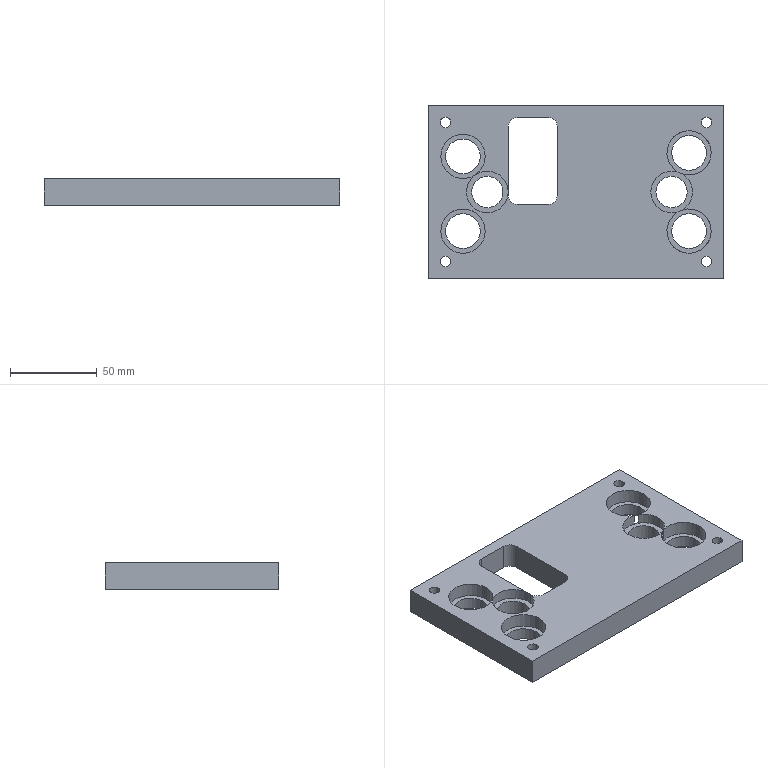Part | STEP file | solid 32 | 1 solid | 37 faces | box 170 x 100 x 15 mm | volume 197483 mm3 | cylinder 21 | plane 16 | commonest cylinder face diameters 6 x4 10 x4 20 x4 25.5 x4 24 x3 18 x2